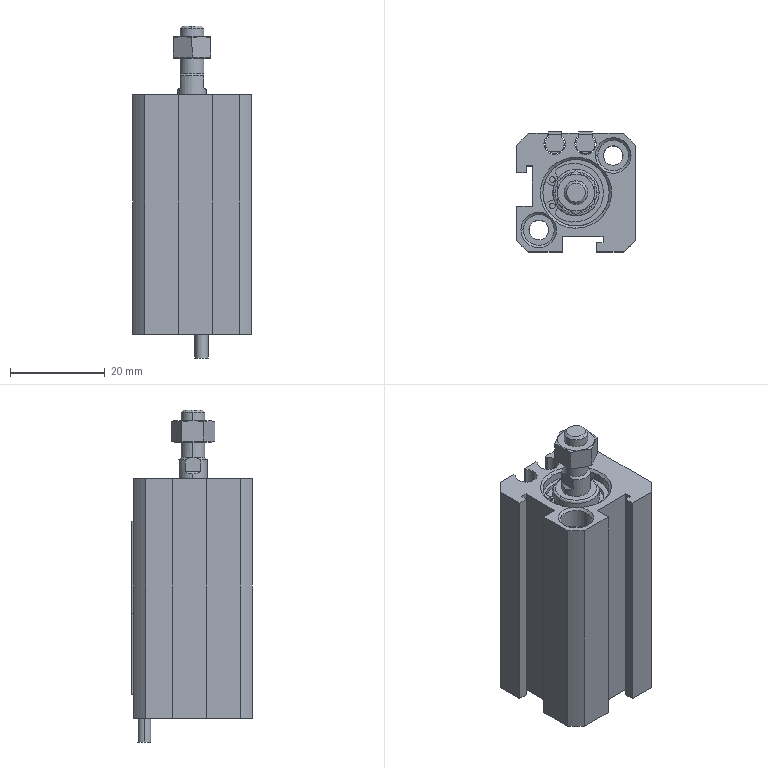Part | SolidWorks | features Attribute 1 | 5 solids | 244 faces | box 25 x 25.4 x 70 mm | volume 23906 mm3 | plane 111 | cylinder 101 | cone 28 | spline 4 | commonest cylinder face diameters 2.4 x14 4.134 x14 1.2 x8 6.5 x8 4 x6 4.5 x6